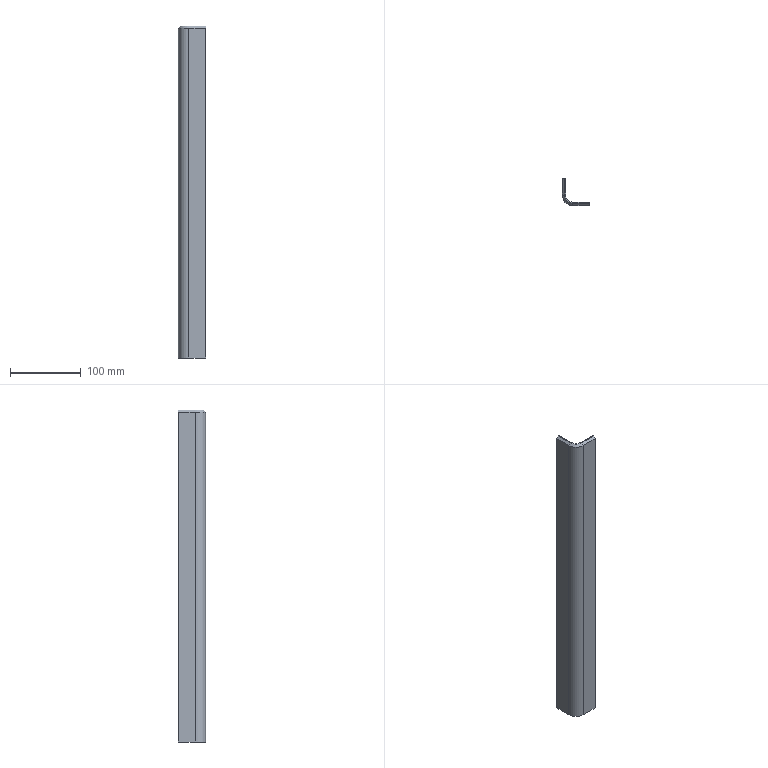Part | SolidWorks | features Chamfer 1, FlatPattern 1, SMBaseFlange 1, SheetMetal 1 | 1 solid | 17 faces | box 38.5 x 38.5 x 470 mm | volume 141906 mm3 | plane 14 | cylinder 2 | cone 1 | commonest cylinder face diameters 20 x1 29 x1
STEP:
#1=CARTESIAN_POINT('',(3.,14.5,235.));
#2=VERTEX_POINT('',#1);
#3=CARTESIAN_POINT('',(4.5,14.5,235.));
#4=VERTEX_POINT('',#3);
#5=CARTESIAN_POINT('',(0.,14.5,235.));
#6=DIRECTION('',(1.,0.,0.));
#7=VECTOR('',#6,1000.);
#8=LINE('',#5,#7);
#9=EDGE_CURVE('',#2,#4,#8,.T.);
#10=ORIENTED_EDGE('',*,*,#9,.F.);
#11=CARTESIAN_POINT('',(14.5,3.,235.));
#12=VERTEX_POINT('',#11);
#13=CARTESIAN_POINT('',(14.5,14.5,235.));
#14=DIRECTION('',(0.,0.,1.));
#15=DIRECTION('',(1.,0.,0.));
#16=AXIS2_PLACEMENT_3D('',#13,#14,#15);
#17=CIRCLE('',#16,11.5);
#18=EDGE_CURVE('',#2,#12,#17,.T.);
#19=ORIENTED_EDGE('',*,*,#18,.T.);
#20=CARTESIAN_POINT('',(14.5,4.5,235.));
#21=VERTEX_POINT('',#20);
#22=CARTESIAN_POINT('',(14.5,4.5,235.));
#23=DIRECTION('',(0.,-1.,0.));
#24=VECTOR('',#23,1000.);
#25=LINE('',#22,#24);
#26=EDGE_CURVE('',#21,#12,#25,.T.);
#27=ORIENTED_EDGE('',*,*,#26,.F.);
#28=CARTESIAN_POINT('',(14.5,14.5,235.));
#29=DIRECTION('',(0.,0.,-1.));
#30=DIRECTION('',(1.,0.,0.));
#31=AXIS2_PLACEMENT_3D('',#28,#29,#30);
#32=CIRCLE('',#31,10.);
#33=EDGE_CURVE('',#21,#4,#32,.T.);
#34=ORIENTED_EDGE('',*,*,#33,.T.);
#35=EDGE_LOOP('',(#10,#19,#27,#34));
#36=FACE_OUTER_BOUND('',#35,.T.);
#37=CARTESIAN_POINT('',(0.,14.5,235.));
#38=DIRECTION('',(0.,0.,1.));
#39=DIRECTION('',(1.,0.,0.));
#40=AXIS2_PLACEMENT_3D('',#37,#38,#39);
#41=PLANE('',#40);
#42=ADVANCED_FACE('',(#36),#41,.T.);
#43=CARTESIAN_POINT('',(3.,38.5,235.));
#44=VERTEX_POINT('',#43);
#45=CARTESIAN_POINT('',(4.5,38.5,235.));
#46=VERTEX_POINT('',#45);
#47=CARTESIAN_POINT('',(0.,38.5,235.));
#48=DIRECTION('',(1.,0.,0.));
#49=VECTOR('',#48,1000.);
#50=LINE('',#47,#49);
#51=EDGE_CURVE('',#44,#46,#50,.T.);
#52=ORIENTED_EDGE('',*,*,#51,.F.);
#53=CARTESIAN_POINT('',(3.,4.5,235.));
#54=DIRECTION('',(0.,-1.,0.));
#55=VECTOR('',#54,1000.);
#56=LINE('',#53,#55);
#57=EDGE_CURVE('',#44,#2,#56,.T.);
#58=ORIENTED_EDGE('',*,*,#57,.T.);
#59=ORIENTED_EDGE('',*,*,#9,.T.);
#60=CARTESIAN_POINT('',(4.5,0.,235.));
#61=DIRECTION('',(0.,1.,0.));
#62=VECTOR('',#61,1000.);
#63=LINE('',#60,#62);
#64=EDGE_CURVE('',#4,#46,#63,.T.);
#65=ORIENTED_EDGE('',*,*,#64,.T.);
#66=EDGE_LOOP('',(#52,#58,#59,#65));
#67=FACE_OUTER_BOUND('',#66,.T.);
#68=CARTESIAN_POINT('',(14.5,4.5,235.));
#69=DIRECTION('',(0.,0.,1.));
#70=DIRECTION('',(1.,0.,0.));
#71=AXIS2_PLACEMENT_3D('',#68,#69,#70);
#72=PLANE('',#71);
#73=ADVANCED_FACE('',(#67),#72,.T.);
#74=CARTESIAN_POINT('',(14.5,0.,-235.));
#75=VERTEX_POINT('',#74);
#76=CARTESIAN_POINT('',(14.5,4.5,-235.));
#77=VERTEX_POINT('',#76);
#78=CARTESIAN_POINT('',(14.5,0.,-235.));
#79=DIRECTION('',(0.,1.,0.));
#80=VECTOR('',#79,1000.);
#81=LINE('',#78,#80);
#82=EDGE_CURVE('',#75,#77,#81,.T.);
#83=ORIENTED_EDGE('',*,*,#82,.F.);
#84=CARTESIAN_POINT('',(0.,14.5,-235.));
#85=VERTEX_POINT('',#84);
#86=CARTESIAN_POINT('',(14.5,14.5,-235.));
#87=DIRECTION('',(0.,0.,-1.));
#88=DIRECTION('',(1.,0.,0.));
#89=AXIS2_PLACEMENT_3D('',#86,#87,#88);
#90=CIRCLE('',#89,14.5);
#91=EDGE_CURVE('',#75,#85,#90,.T.);
#92=ORIENTED_EDGE('',*,*,#91,.T.);
#93=CARTESIAN_POINT('',(4.5,14.5,-235.));
#94=VERTEX_POINT('',#93);
#95=CARTESIAN_POINT('',(4.5,14.5,-235.));
#96=DIRECTION('',(-1.,0.,0.));
#97=VECTOR('',#96,1000.);
#98=LINE('',#95,#97);
#99=EDGE_CURVE('',#94,#85,#98,.T.);
#100=ORIENTED_EDGE('',*,*,#99,.F.);
#101=CARTESIAN_POINT('',(14.5,14.5,-235.));
#102=DIRECTION('',(0.,0.,-1.));
#103=DIRECTION('',(1.,0.,0.));
#104=AXIS2_PLACEMENT_3D('',#101,#102,#103);
#105=CIRCLE('',#104,10.);
#106=EDGE_CURVE('',#77,#94,#105,.T.);
#107=ORIENTED_EDGE('',*,*,#106,.F.);
#108=EDGE_LOOP('',(#83,#92,#100,#107));
#109=FACE_OUTER_BOUND('',#108,.T.);
#110=CARTESIAN_POINT('',(14.5,0.,-235.));
#111=DIRECTION('',(0.,0.,-1.));
#112=DIRECTION('',(-1.,0.,0.));
#113=AXIS2_PLACEMENT_3D('',#110,#111,#112);
#114=PLANE('',#113);
#115=ADVANCED_FACE('',(#109),#114,.T.);
#116=CARTESIAN_POINT('',(38.5,0.,-235.));
#117=VERTEX_POINT('',#116);
#118=CARTESIAN_POINT('',(0.,0.,-235.));
#119=DIRECTION('',(-1.,0.,0.));
#120=VECTOR('',#119,1000.);
#121=LINE('',#118,#120);
#122=EDGE_CURVE('',#117,#75,#121,.T.);
#123=ORIENTED_EDGE('',*,*,#122,.T.);
#124=ORIENTED_EDGE('',*,*,#82,.T.);
#125=CARTESIAN_POINT('',(38.5,4.5,-235.));
#126=VERTEX_POINT('',#125);
#127=CARTESIAN_POINT('',(0.,4.5,-235.));
#128=DIRECTION('',(-1.,0.,0.));
#129=VECTOR('',#128,1000.);
#130=LINE('',#127,#129);
#131=EDGE_CURVE('',#126,#77,#130,.T.);
#132=ORIENTED_EDGE('',*,*,#131,.F.);
#133=CARTESIAN_POINT('',(38.5,4.5,-235.));
#134=DIRECTION('',(0.,-1.,0.));
#135=VECTOR('',#134,1000.);
#136=LINE('',#133,#135);
#137=EDGE_CURVE('',#126,#117,#136,.T.);
#138=ORIENTED_EDGE('',*,*,#137,.T.);
#139=EDGE_LOOP('',(#123,#124,#132,#138));
#140=FACE_OUTER_BOUND('',#139,.T.);
#141=CARTESIAN_POINT('',(4.5,14.5,-235.));
#142=DIRECTION('',(0.,0.,-1.));
#143=DIRECTION('',(-1.,0.,0.));
#144=AXIS2_PLACEMENT_3D('',#141,#142,#143);
#145=PLANE('',#144);
#146=ADVANCED_FACE('',(#140),#145,.T.);
#147=CARTESIAN_POINT('',(4.5,38.5,-235.));
#148=VERTEX_POINT('',#147);
#149=CARTESIAN_POINT('',(4.5,0.,-235.));
#150=DIRECTION('',(0.,1.,0.));
#151=VECTOR('',#150,1000.);
#152=LINE('',#149,#151);
#153=EDGE_CURVE('',#94,#148,#152,.T.);
#154=ORIENTED_EDGE('',*,*,#153,.T.);
#155=CARTESIAN_POINT('',(4.5,38.5,235.));
#156=DIRECTION('',(0.,0.,-1.));
#157=VECTOR('',#156,1000.);
#158=LINE('',#155,#157);
#159=EDGE_CURVE('',#46,#148,#158,.T.);
#160=ORIENTED_EDGE('',*,*,#159,.F.);
#161=ORIENTED_EDGE('',*,*,#64,.F.);
#162=CARTESIAN_POINT('',(4.5,14.5,235.));
#163=DIRECTION('',(0.,0.,-1.));
#164=VECTOR('',#163,1000.);
#165=LINE('',#162,#164);
#166=EDGE_CURVE('',#4,#94,#165,.T.);
#167=ORIENTED_EDGE('',*,*,#166,.T.);
#168=EDGE_LOOP('',(#154,#160,#161,#167));
#169=FACE_OUTER_BOUND('',#168,.T.);
#170=CARTESIAN_POINT('',(4.5,0.,235.));
#171=DIRECTION('',(-1.,0.,0.));
#172=DIRECTION('',(0.,0.,1.));
#173=AXIS2_PLACEMENT_3D('',#170,#171,#172);
#174=PLANE('',#173);
#175=ADVANCED_FACE('',(#169),#174,.F.);
#176=CARTESIAN_POINT('',(0.,38.5,232.));
#177=VERTEX_POINT('',#176);
#178=CARTESIAN_POINT('',(0.,38.5,-235.));
#179=VERTEX_POINT('',#178);
#180=CARTESIAN_POINT('',(0.,38.5,235.));
#181=DIRECTION('',(0.,0.,-1.));
#182=VECTOR('',#181,1000.);
#183=LINE('',#180,#182);
#184=EDGE_CURVE('',#177,#179,#183,.T.);
#185=ORIENTED_EDGE('',*,*,#184,.F.);
#186=CARTESIAN_POINT('',(1.5,38.5,233.5));
#187=DIRECTION('',(0.7071,0.,0.7071));
#188=VECTOR('',#187,1000.);
#189=LINE('',#186,#188);
#190=EDGE_CURVE('',#177,#44,#189,.T.);
#191=ORIENTED_EDGE('',*,*,#190,.T.);
#192=ORIENTED_EDGE('',*,*,#51,.T.);
#193=ORIENTED_EDGE('',*,*,#159,.T.);
#194=CARTESIAN_POINT('',(0.,38.5,-235.));
#195=DIRECTION('',(1.,0.,0.));
#196=VECTOR('',#195,1000.);
#197=LINE('',#194,#196);
#198=EDGE_CURVE('',#179,#148,#197,.T.);
#199=ORIENTED_EDGE('',*,*,#198,.F.);
#200=EDGE_LOOP('',(#185,#191,#192,#193,#199));
#201=FACE_OUTER_BOUND('',#200,.T.);
#202=CARTESIAN_POINT('',(0.,38.5,235.));
#203=DIRECTION('',(0.,1.,0.));
#204=DIRECTION('',(0.,0.,1.));
#205=AXIS2_PLACEMENT_3D('',#202,#203,#204);
#206=PLANE('',#205);
#207=ADVANCED_FACE('',(#201),#206,.T.);
#208=CARTESIAN_POINT('',(0.,14.5,232.));
#209=VERTEX_POINT('',#208);
#210=CARTESIAN_POINT('',(0.,14.5,235.));
#211=DIRECTION('',(0.,0.,-1.));
#212=VECTOR('',#211,1000.);
#213=LINE('',#210,#212);
#214=EDGE_CURVE('',#209,#85,#213,.T.);
#215=ORIENTED_EDGE('',*,*,#214,.F.);
#216=CARTESIAN_POINT('',(0.,0.,232.));
#217=DIRECTION('',(0.,1.,0.));
#218=VECTOR('',#217,1000.);
#219=LINE('',#216,#218);
#220=EDGE_CURVE('',#209,#177,#219,.T.);
#221=ORIENTED_EDGE('',*,*,#220,.T.);
#222=ORIENTED_EDGE('',*,*,#184,.T.);
#223=CARTESIAN_POINT('',(0.,0.,-235.));
#224=DIRECTION('',(0.,1.,0.));
#225=VECTOR('',#224,1000.);
#226=LINE('',#223,#225);
#227=EDGE_CURVE('',#85,#179,#226,.T.);
#228=ORIENTED_EDGE('',*,*,#227,.F.);
#229=EDGE_LOOP('',(#215,#221,#222,#228));
#230=FACE_OUTER_BOUND('',#229,.T.);
#231=CARTESIAN_POINT('',(0.,0.,235.));
#232=DIRECTION('',(-1.,0.,0.));
#233=DIRECTION('',(0.,0.,1.));
#234=AXIS2_PLACEMENT_3D('',#231,#232,#233);
#235=PLANE('',#234);
#236=ADVANCED_FACE('',(#230),#235,.T.);
#237=CARTESIAN_POINT('',(14.5,0.,232.));
#238=VERTEX_POINT('',#237);
#239=CARTESIAN_POINT('',(14.5,0.,235.));
#240=DIRECTION('',(0.,0.,-1.));
#241=VECTOR('',#240,1000.);
#242=LINE('',#239,#241);
#243=EDGE_CURVE('',#238,#75,#242,.T.);
#244=ORIENTED_EDGE('',*,*,#243,.F.);
#245=CARTESIAN_POINT('',(14.5,14.5,232.));
#246=DIRECTION('',(0.,0.,-1.));
#247=DIRECTION('',(1.,0.,0.));
#248=AXIS2_PLACEMENT_3D('',#245,#246,#247);
#249=CIRCLE('',#248,14.5);
#250=EDGE_CURVE('',#238,#209,#249,.T.);
#251=ORIENTED_EDGE('',*,*,#250,.T.);
#252=ORIENTED_EDGE('',*,*,#214,.T.);
#253=ORIENTED_EDGE('',*,*,#91,.F.);
#254=EDGE_LOOP('',(#244,#251,#252,#253));
#255=FACE_OUTER_BOUND('',#254,.T.);
#256=CARTESIAN_POINT('',(14.5,14.5,235.));
#257=DIRECTION('',(0.,0.,-1.));
#258=DIRECTION('',(-1.,0.,0.));
#259=AXIS2_PLACEMENT_3D('',#256,#257,#258);
#260=CYLINDRICAL_SURFACE('',#259,14.5);
#261=ADVANCED_FACE('',(#255),#260,.T.);
#262=CARTESIAN_POINT('',(38.5,0.,232.));
#263=VERTEX_POINT('',#262);
#264=CARTESIAN_POINT('',(38.5,0.,235.));
#265=DIRECTION('',(0.,0.,-1.));
#266=VECTOR('',#265,1000.);
#267=LINE('',#264,#266);
#268=EDGE_CURVE('',#263,#117,#267,.T.);
#269=ORIENTED_EDGE('',*,*,#268,.F.);
#270=CARTESIAN_POINT('',(0.,0.,232.));
#271=DIRECTION('',(-1.,0.,0.));
#272=VECTOR('',#271,1000.);
#273=LINE('',#270,#272);
#274=EDGE_CURVE('',#263,#238,#273,.T.);
#275=ORIENTED_EDGE('',*,*,#274,.T.);
#276=ORIENTED_EDGE('',*,*,#243,.T.);
#277=ORIENTED_EDGE('',*,*,#122,.F.);
#278=EDGE_LOOP('',(#269,#275,#276,#277));
#279=FACE_OUTER_BOUND('',#278,.T.);
#280=CARTESIAN_POINT('',(0.,0.,235.));
#281=DIRECTION('',(0.,-1.,0.));
#282=DIRECTION('',(0.,0.,-1.));
#283=AXIS2_PLACEMENT_3D('',#280,#281,#282);
#284=PLANE('',#283);
#285=ADVANCED_FACE('',(#279),#284,.T.);
#286=CARTESIAN_POINT('',(38.5,4.5,235.));
#287=VERTEX_POINT('',#286);
#288=CARTESIAN_POINT('',(38.5,3.,235.));
#289=VERTEX_POINT('',#288);
#290=CARTESIAN_POINT('',(38.5,4.5,235.));
#291=DIRECTION('',(0.,-1.,0.));
#292=VECTOR('',#291,1000.);
#293=LINE('',#290,#292);
#294=EDGE_CURVE('',#287,#289,#293,.T.);
#295=ORIENTED_EDGE('',*,*,#294,.T.);
#296=CARTESIAN_POINT('',(38.5,3.75,235.75));
#297=DIRECTION('',(0.,-0.7071,-0.7071));
#298=VECTOR('',#297,1000.);
#299=LINE('',#296,#298);
#300=EDGE_CURVE('',#289,#263,#299,.T.);
#301=ORIENTED_EDGE('',*,*,#300,.T.);
#302=ORIENTED_EDGE('',*,*,#268,.T.);
#303=ORIENTED_EDGE('',*,*,#137,.F.);
#304=CARTESIAN_POINT('',(38.5,4.5,235.));
#305=DIRECTION('',(0.,0.,-1.));
#306=VECTOR('',#305,1000.);
#307=LINE('',#304,#306);
#308=EDGE_CURVE('',#287,#126,#307,.T.);
#309=ORIENTED_EDGE('',*,*,#308,.F.);
#310=EDGE_LOOP('',(#295,#301,#302,#303,#309));
#311=FACE_OUTER_BOUND('',#310,.T.);
#312=CARTESIAN_POINT('',(38.5,4.5,235.));
#313=DIRECTION('',(1.,0.,0.));
#314=DIRECTION('',(0.,0.,-1.));
#315=AXIS2_PLACEMENT_3D('',#312,#313,#314);
#316=PLANE('',#315);
#317=ADVANCED_FACE('',(#311),#316,.T.);
#318=ORIENTED_EDGE('',*,*,#131,.T.);
#319=CARTESIAN_POINT('',(14.5,4.5,235.));
#320=DIRECTION('',(0.,0.,-1.));
#321=VECTOR('',#320,1000.);
#322=LINE('',#319,#321);
#323=EDGE_CURVE('',#21,#77,#322,.T.);
#324=ORIENTED_EDGE('',*,*,#323,.F.);
#325=CARTESIAN_POINT('',(0.,4.5,235.));
#326=DIRECTION('',(-1.,0.,0.));
#327=VECTOR('',#326,1000.);
#328=LINE('',#325,#327);
#329=EDGE_CURVE('',#287,#21,#328,.T.);
#330=ORIENTED_EDGE('',*,*,#329,.F.);
#331=ORIENTED_EDGE('',*,*,#308,.T.);
#332=EDGE_LOOP('',(#318,#324,#330,#331));
#333=FACE_OUTER_BOUND('',#332,.T.);
#334=CARTESIAN_POINT('',(0.,4.5,235.));
#335=DIRECTION('',(0.,-1.,0.));
#336=DIRECTION('',(0.,0.,-1.));
#337=AXIS2_PLACEMENT_3D('',#334,#335,#336);
#338=PLANE('',#337);
#339=ADVANCED_FACE('',(#333),#338,.F.);
#340=ORIENTED_EDGE('',*,*,#106,.T.);
#341=ORIENTED_EDGE('',*,*,#166,.F.);
#342=ORIENTED_EDGE('',*,*,#33,.F.);
#343=ORIENTED_EDGE('',*,*,#323,.T.);
#344=EDGE_LOOP('',(#340,#341,#342,#343));
#345=FACE_OUTER_BOUND('',#344,.T.);
#346=CARTESIAN_POINT('',(14.5,14.5,235.));
#347=DIRECTION('',(0.,0.,-1.));
#348=DIRECTION('',(-1.,0.,0.));
#349=AXIS2_PLACEMENT_3D('',#346,#347,#348);
#350=CYLINDRICAL_SURFACE('',#349,10.);
#351=ADVANCED_FACE('',(#345),#350,.F.);
#352=ORIENTED_EDGE('',*,*,#26,.T.);
#353=CARTESIAN_POINT('',(14.5,3.,235.));
#354=DIRECTION('',(1.,0.,0.));
#355=VECTOR('',#354,1000.);
#356=LINE('',#353,#355);
#357=EDGE_CURVE('',#12,#289,#356,.T.);
#358=ORIENTED_EDGE('',*,*,#357,.T.);
#359=ORIENTED_EDGE('',*,*,#294,.F.);
#360=ORIENTED_EDGE('',*,*,#329,.T.);
#361=EDGE_LOOP('',(#352,#358,#359,#360));
#362=FACE_OUTER_BOUND('',#361,.T.);
#363=CARTESIAN_POINT('',(14.5,14.5,235.));
#364=DIRECTION('',(0.,0.,1.));
#365=DIRECTION('',(1.,0.,0.));
#366=AXIS2_PLACEMENT_3D('',#363,#364,#365);
#367=PLANE('',#366);
#368=ADVANCED_FACE('',(#362),#367,.T.);
#369=ORIENTED_EDGE('',*,*,#153,.F.);
#370=ORIENTED_EDGE('',*,*,#99,.T.);
#371=ORIENTED_EDGE('',*,*,#227,.T.);
#372=ORIENTED_EDGE('',*,*,#198,.T.);
#373=EDGE_LOOP('',(#369,#370,#371,#372));
#374=FACE_OUTER_BOUND('',#373,.T.);
#375=CARTESIAN_POINT('',(14.5,14.5,-235.));
#376=DIRECTION('',(0.,0.,1.));
#377=DIRECTION('',(1.,0.,0.));
#378=AXIS2_PLACEMENT_3D('',#375,#376,#377);
#379=PLANE('',#378);
#380=ADVANCED_FACE('',(#374),#379,.F.);
#381=ORIENTED_EDGE('',*,*,#190,.F.);
#382=ORIENTED_EDGE('',*,*,#220,.F.);
#383=CARTESIAN_POINT('',(3.,14.5,235.));
#384=DIRECTION('',(-0.7071,0.,-0.7071));
#385=VECTOR('',#384,1000.);
#386=LINE('',#383,#385);
#387=EDGE_CURVE('',#2,#209,#386,.T.);
#388=ORIENTED_EDGE('',*,*,#387,.F.);
#389=ORIENTED_EDGE('',*,*,#57,.F.);
#390=EDGE_LOOP('',(#381,#382,#388,#389));
#391=FACE_OUTER_BOUND('',#390,.T.);
#392=CARTESIAN_POINT('',(0.,0.,232.));
#393=DIRECTION('',(0.7071,0.,-0.7071));
#394=DIRECTION('',(0.,1.,0.));
#395=AXIS2_PLACEMENT_3D('',#392,#393,#394);
#396=PLANE('',#395);
#397=ADVANCED_FACE('',(#391),#396,.F.);
#398=ORIENTED_EDGE('',*,*,#387,.T.);
#399=ORIENTED_EDGE('',*,*,#250,.F.);
#400=CARTESIAN_POINT('',(14.5,3.,235.));
#401=DIRECTION('',(0.,-0.7071,-0.7071));
#402=VECTOR('',#401,1000.);
#403=LINE('',#400,#402);
#404=EDGE_CURVE('',#12,#238,#403,.T.);
#405=ORIENTED_EDGE('',*,*,#404,.F.);
#406=ORIENTED_EDGE('',*,*,#18,.F.);
#407=EDGE_LOOP('',(#398,#399,#405,#406));
#408=FACE_OUTER_BOUND('',#407,.T.);
#409=CARTESIAN_POINT('',(14.5,14.5,232.));
#410=DIRECTION('',(0.,0.,-1.));
#411=DIRECTION('',(-1.,0.,0.));
#412=AXIS2_PLACEMENT_3D('',#409,#410,#411);
#413=CONICAL_SURFACE('',#412,14.5,0.7854);
#414=ADVANCED_FACE('',(#408),#413,.T.);
#415=ORIENTED_EDGE('',*,*,#300,.F.);
#416=ORIENTED_EDGE('',*,*,#357,.F.);
#417=ORIENTED_EDGE('',*,*,#404,.T.);
#418=ORIENTED_EDGE('',*,*,#274,.F.);
#419=EDGE_LOOP('',(#415,#416,#417,#418));
#420=FACE_OUTER_BOUND('',#419,.T.);
#421=CARTESIAN_POINT('',(0.,0.,232.));
#422=DIRECTION('',(0.,0.7071,-0.7071));
#423=DIRECTION('',(-1.,0.,0.));
#424=AXIS2_PLACEMENT_3D('',#421,#422,#423);
#425=PLANE('',#424);
#426=ADVANCED_FACE('',(#420),#425,.F.);
#427=CLOSED_SHELL('',(#42,#73,#115,#146,#175,#207,#236,#261,#285,#317,#339,#351,#368,#380,#397,#414,#426));
#428=MANIFOLD_SOLID_BREP('',#427);
#429=CARTESIAN_POINT('',(0.,0.,0.));
#430=DIRECTION('',(0.,0.,1.));
#431=DIRECTION('',(1.,0.,0.));
#432=AXIS2_PLACEMENT_3D('',#429,#430,#431);
#433=(LENGTH_UNIT()NAMED_UNIT(*)SI_UNIT(.MILLI.,.METRE.));
#434=UNCERTAINTY_MEASURE_WITH_UNIT(LENGTH_MEASURE(0.00001),#433,'','');
#435=(NAMED_UNIT(*)PLANE_ANGLE_UNIT()SI_UNIT($,.RADIAN.));
#436=(NAMED_UNIT(*)SI_UNIT($,.STERADIAN.)SOLID_ANGLE_UNIT());
#437=(GEOMETRIC_REPRESENTATION_CONTEXT(3)GLOBAL_UNCERTAINTY_ASSIGNED_CONTEXT((#434))GLOBAL_UNIT_ASSIGNED_CONTEXT((#433,#435,#436))REPRESENTATION_CONTEXT('',''));
#438=ADVANCED_BREP_SHAPE_REPRESENTATION('',(#428,#432),#437);